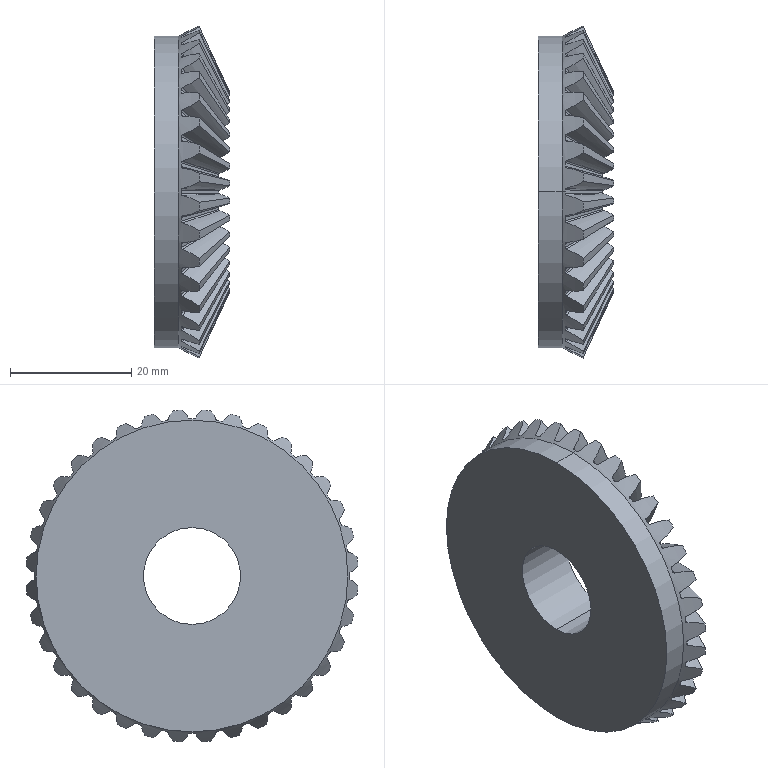Part | SolidWorks | features CirPattern 2, Cut 2, BlendCut 1, Boss 1, ICE 1, Revolution 1 | 1 solid | 226 faces | box 12.396 x 54.775 x 54.775 mm | volume 17958 mm3 | spline 180 | cone 40 | cylinder 4 | plane 2 | commonest cylinder face diameters 16 x2 51.428 x2